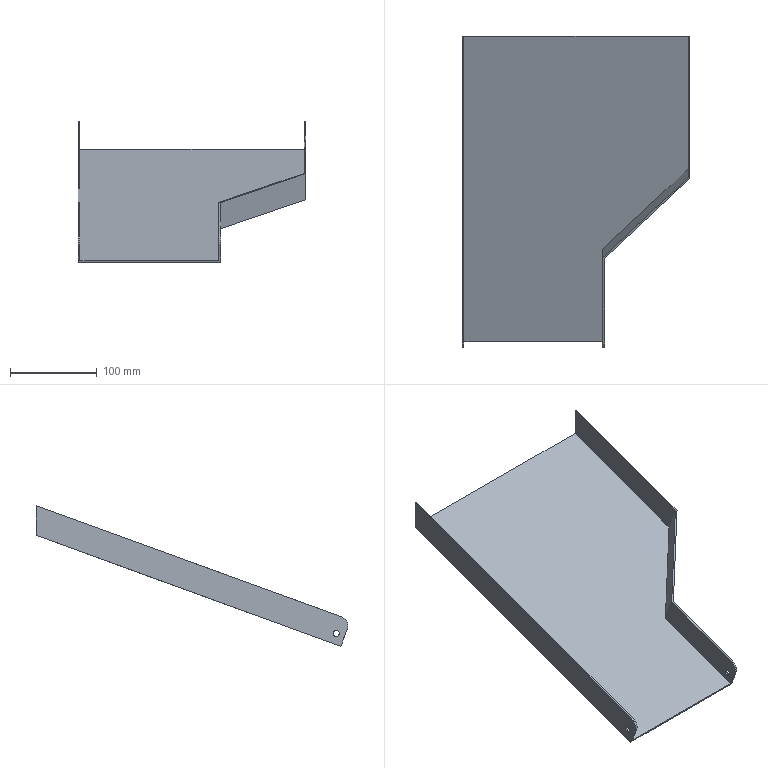Part | NX | features HB 2 | 1 solid | 18 faces | box 262 x 359.033 x 161.773 mm | volume 211954 mm3 | plane 14 | cylinder 4 | commonest cylinder face diameters 7 x2 20 x2
STEP:
#1=CARTESIAN_POINT('',(122.,-585.061,-351.381));
#2=VERTEX_POINT('',#1);
#3=CARTESIAN_POINT('',(122.,-691.589,-390.154));
#4=VERTEX_POINT('',#3);
#5=CARTESIAN_POINT('',(122.,-379.611,-276.603));
#6=DIRECTION('',(0.,-0.9397,-0.342));
#7=VECTOR('',#6,1000.);
#8=LINE('',#5,#7);
#9=EDGE_CURVE('',#2,#4,#8,.T.);
#10=ORIENTED_EDGE('',*,*,#9,.F.);
#11=CARTESIAN_POINT('',(220.,-492.971,-317.863));
#12=VERTEX_POINT('',#11);
#13=CARTESIAN_POINT('',(261.318,-454.145,-303.731));
#14=DIRECTION('',(-0.7071,-0.6645,-0.2418));
#15=VECTOR('',#14,1000.);
#16=LINE('',#13,#15);
#17=EDGE_CURVE('',#12,#2,#16,.T.);
#18=ORIENTED_EDGE('',*,*,#17,.F.);
#19=CARTESIAN_POINT('',(220.,-340.,-262.186));
#20=VERTEX_POINT('',#19);
#21=CARTESIAN_POINT('',(220.,-379.611,-276.603));
#22=DIRECTION('',(0.,-0.9397,-0.342));
#23=VECTOR('',#22,1000.);
#24=LINE('',#21,#23);
#25=EDGE_CURVE('',#20,#12,#24,.T.);
#26=ORIENTED_EDGE('',*,*,#25,.F.);
#27=CARTESIAN_POINT('',(-38.,-340.,-262.186));
#28=VERTEX_POINT('',#27);
#29=CARTESIAN_POINT('',(182.,-340.,-262.186));
#30=DIRECTION('',(-1.,0.,0.));
#31=VECTOR('',#30,1000.);
#32=LINE('',#29,#31);
#33=EDGE_CURVE('',#20,#28,#32,.T.);
#34=ORIENTED_EDGE('',*,*,#33,.T.);
#35=CARTESIAN_POINT('',(-38.,-691.589,-390.154));
#36=VERTEX_POINT('',#35);
#37=CARTESIAN_POINT('',(-38.,-379.611,-276.603));
#38=DIRECTION('',(0.,0.9397,0.342));
#39=VECTOR('',#38,1000.);
#40=LINE('',#37,#39);
#41=EDGE_CURVE('',#36,#28,#40,.T.);
#42=ORIENTED_EDGE('',*,*,#41,.F.);
#43=CARTESIAN_POINT('',(182.,-691.589,-390.154));
#44=DIRECTION('',(1.,0.,0.));
#45=VECTOR('',#44,1000.);
#46=LINE('',#43,#45);
#47=EDGE_CURVE('',#36,#4,#46,.T.);
#48=ORIENTED_EDGE('',*,*,#47,.T.);
#49=EDGE_LOOP('',(#10,#18,#26,#34,#42,#48));
#50=FACE_BOUND('',#49,.T.);
#51=CARTESIAN_POINT('',(182.,-379.611,-276.603));
#52=DIRECTION('',(0.,-0.342,0.9397));
#53=DIRECTION('',(-1.,0.,0.));
#54=AXIS2_PLACEMENT_3D('',#51,#52,#53);
#55=PLANE('',#54);
#56=ADVANCED_FACE('',(#50),#55,.T.);
#57=CARTESIAN_POINT('',(220.,-340.,-230.26));
#58=VERTEX_POINT('',#57);
#59=CARTESIAN_POINT('',(222.,-340.,-230.26));
#60=VERTEX_POINT('',#59);
#61=CARTESIAN_POINT('',(222.,-340.,-230.26));
#62=DIRECTION('',(1.,0.,0.));
#63=VECTOR('',#62,1000.);
#64=LINE('',#61,#63);
#65=EDGE_CURVE('',#58,#60,#64,.T.);
#66=ORIENTED_EDGE('',*,*,#65,.T.);
#67=CARTESIAN_POINT('',(222.,-340.,-264.314));
#68=VERTEX_POINT('',#67);
#69=CARTESIAN_POINT('',(222.,-340.,-276.603));
#70=DIRECTION('',(0.,0.,-1.));
#71=VECTOR('',#70,1000.);
#72=LINE('',#69,#71);
#73=EDGE_CURVE('',#60,#68,#72,.T.);
#74=ORIENTED_EDGE('',*,*,#73,.T.);
#75=CARTESIAN_POINT('',(-40.,-340.,-264.314));
#76=VERTEX_POINT('',#75);
#77=CARTESIAN_POINT('',(182.,-340.,-264.314));
#78=DIRECTION('',(-1.,0.,0.));
#79=VECTOR('',#78,1000.);
#80=LINE('',#77,#79);
#81=EDGE_CURVE('',#68,#76,#80,.T.);
#82=ORIENTED_EDGE('',*,*,#81,.T.);
#83=CARTESIAN_POINT('',(-40.,-340.,-230.26));
#84=VERTEX_POINT('',#83);
#85=CARTESIAN_POINT('',(-40.,-340.,-276.603));
#86=DIRECTION('',(0.,0.,1.));
#87=VECTOR('',#86,1000.);
#88=LINE('',#85,#87);
#89=EDGE_CURVE('',#76,#84,#88,.T.);
#90=ORIENTED_EDGE('',*,*,#89,.T.);
#91=CARTESIAN_POINT('',(-38.,-340.,-230.26));
#92=VERTEX_POINT('',#91);
#93=CARTESIAN_POINT('',(-48.,-340.,-230.26));
#94=DIRECTION('',(1.,0.,0.));
#95=VECTOR('',#94,1000.);
#96=LINE('',#93,#95);
#97=EDGE_CURVE('',#84,#92,#96,.T.);
#98=ORIENTED_EDGE('',*,*,#97,.T.);
#99=CARTESIAN_POINT('',(-38.,-340.,-276.603));
#100=DIRECTION('',(0.,0.,1.));
#101=VECTOR('',#100,1000.);
#102=LINE('',#99,#101);
#103=EDGE_CURVE('',#28,#92,#102,.T.);
#104=ORIENTED_EDGE('',*,*,#103,.F.);
#105=ORIENTED_EDGE('',*,*,#33,.F.);
#106=CARTESIAN_POINT('',(220.,-340.,-276.603));
#107=DIRECTION('',(0.,0.,-1.));
#108=VECTOR('',#107,1000.);
#109=LINE('',#106,#108);
#110=EDGE_CURVE('',#58,#20,#109,.T.);
#111=ORIENTED_EDGE('',*,*,#110,.F.);
#112=EDGE_LOOP('',(#66,#74,#82,#90,#98,#104,#105,#111));
#113=FACE_BOUND('',#112,.T.);
#114=CARTESIAN_POINT('',(-210.,-340.,60.));
#115=DIRECTION('',(0.,1.,0.));
#116=DIRECTION('',(0.,0.,-1.));
#117=AXIS2_PLACEMENT_3D('',#114,#115,#116);
#118=PLANE('',#117);
#119=ADVANCED_FACE('',(#113),#118,.T.);
#120=CARTESIAN_POINT('',(220.,-503.232,-289.672));
#121=VERTEX_POINT('',#120);
#122=CARTESIAN_POINT('',(220.,-492.971,-317.863));
#123=DIRECTION('',(0.,0.342,-0.9397));
#124=VECTOR('',#123,1000.);
#125=LINE('',#122,#124);
#126=EDGE_CURVE('',#121,#12,#125,.T.);
#127=ORIENTED_EDGE('',*,*,#126,.F.);
#128=CARTESIAN_POINT('',(220.,-389.872,-248.412));
#129=DIRECTION('',(0.,-0.9397,-0.342));
#130=VECTOR('',#129,1000.);
#131=LINE('',#128,#130);
#132=EDGE_CURVE('',#58,#121,#131,.T.);
#133=ORIENTED_EDGE('',*,*,#132,.F.);
#134=ORIENTED_EDGE('',*,*,#110,.T.);
#135=ORIENTED_EDGE('',*,*,#25,.T.);
#136=EDGE_LOOP('',(#127,#133,#134,#135));
#137=FACE_BOUND('',#136,.T.);
#138=CARTESIAN_POINT('',(220.,-379.611,-276.603));
#139=DIRECTION('',(-1.,0.,0.));
#140=DIRECTION('',(0.,0.08716,0.9962));
#141=AXIS2_PLACEMENT_3D('',#138,#139,#140);
#142=PLANE('',#141);
#143=ADVANCED_FACE('',(#137),#142,.T.);
#144=CARTESIAN_POINT('',(-40.,-690.905,-392.033));
#145=VERTEX_POINT('',#144);
#146=CARTESIAN_POINT('',(-40.,-378.927,-278.482));
#147=DIRECTION('',(0.,-0.9397,-0.342));
#148=VECTOR('',#147,1000.);
#149=LINE('',#146,#148);
#150=EDGE_CURVE('',#76,#145,#149,.T.);
#151=ORIENTED_EDGE('',*,*,#150,.T.);
#152=CARTESIAN_POINT('',(-40.,-698.43,-371.36));
#153=VERTEX_POINT('',#152);
#154=CARTESIAN_POINT('',(-40.,-691.589,-390.154));
#155=DIRECTION('',(0.,0.342,-0.9397));
#156=VECTOR('',#155,1000.);
#157=LINE('',#154,#156);
#158=EDGE_CURVE('',#153,#145,#157,.T.);
#159=ORIENTED_EDGE('',*,*,#158,.F.);
#160=CARTESIAN_POINT('',(-40.,-692.453,-358.543));
#161=VERTEX_POINT('',#160);
#162=CARTESIAN_POINT('',(-40.,-689.033,-367.939));
#163=DIRECTION('',(-1.,0.,0.));
#164=DIRECTION('',(0.,0.,-1.));
#165=AXIS2_PLACEMENT_3D('',#162,#163,#164);
#166=CIRCLE('',#165,10.);
#167=EDGE_CURVE('',#153,#161,#166,.T.);
#168=ORIENTED_EDGE('',*,*,#167,.T.);
#169=CARTESIAN_POINT('',(-40.,-389.872,-248.412));
#170=DIRECTION('',(0.,-0.9397,-0.342));
#171=VECTOR('',#170,1000.);
#172=LINE('',#169,#171);
#173=EDGE_CURVE('',#84,#161,#172,.T.);
#174=ORIENTED_EDGE('',*,*,#173,.F.);
#175=ORIENTED_EDGE('',*,*,#89,.F.);
#176=EDGE_LOOP('',(#151,#159,#168,#174,#175));
#177=FACE_BOUND('',#176,.T.);
#178=CARTESIAN_POINT('',(-40.,-685.612,-380.836));
#179=VERTEX_POINT('',#178);
#180=CARTESIAN_POINT('',(-40.,-685.612,-377.336));
#181=DIRECTION('',(1.,0.,0.));
#182=DIRECTION('',(0.,0.,-1.));
#183=AXIS2_PLACEMENT_3D('',#180,#181,#182);
#184=CIRCLE('',#183,3.5);
#185=EDGE_CURVE('',#179,#179,#184,.T.);
#186=ORIENTED_EDGE('',*,*,#185,.T.);
#187=EDGE_LOOP('',(#186));
#188=FACE_BOUND('',#187,.T.);
#189=CARTESIAN_POINT('',(-40.,-379.611,-276.603));
#190=DIRECTION('',(1.,0.,0.));
#191=DIRECTION('',(0.,0.08716,0.9962));
#192=AXIS2_PLACEMENT_3D('',#189,#190,#191);
#193=PLANE('',#192);
#194=ADVANCED_FACE('',(#177,#188),#193,.F.);
#195=ORIENTED_EDGE('',*,*,#173,.T.);
#196=CARTESIAN_POINT('',(-38.,-692.453,-358.543));
#197=VERTEX_POINT('',#196);
#198=CARTESIAN_POINT('',(7.,-692.453,-358.543));
#199=DIRECTION('',(1.,0.,0.));
#200=VECTOR('',#199,1000.);
#201=LINE('',#198,#200);
#202=EDGE_CURVE('',#161,#197,#201,.T.);
#203=ORIENTED_EDGE('',*,*,#202,.T.);
#204=CARTESIAN_POINT('',(-38.,-389.872,-248.412));
#205=DIRECTION('',(0.,-0.9397,-0.342));
#206=VECTOR('',#205,1000.);
#207=LINE('',#204,#206);
#208=EDGE_CURVE('',#92,#197,#207,.T.);
#209=ORIENTED_EDGE('',*,*,#208,.F.);
#210=ORIENTED_EDGE('',*,*,#97,.F.);
#211=EDGE_LOOP('',(#195,#203,#209,#210));
#212=FACE_BOUND('',#211,.T.);
#213=CARTESIAN_POINT('',(-48.,-389.872,-248.412));
#214=DIRECTION('',(0.,0.342,-0.9397));
#215=DIRECTION('',(0.,-0.9397,-0.342));
#216=AXIS2_PLACEMENT_3D('',#213,#214,#215);
#217=PLANE('',#216);
#218=ADVANCED_FACE('',(#212),#217,.F.);
#219=CARTESIAN_POINT('',(222.,-493.066,-320.025));
#220=VERTEX_POINT('',#219);
#221=CARTESIAN_POINT('',(124.,-585.156,-353.543));
#222=VERTEX_POINT('',#221);
#223=CARTESIAN_POINT('',(262.732,-454.79,-306.094));
#224=DIRECTION('',(-0.7071,-0.6645,-0.2418));
#225=VECTOR('',#224,1000.);
#226=LINE('',#223,#225);
#227=EDGE_CURVE('',#220,#222,#226,.T.);
#228=ORIENTED_EDGE('',*,*,#227,.T.);
#229=CARTESIAN_POINT('',(124.,-690.905,-392.033));
#230=VERTEX_POINT('',#229);
#231=CARTESIAN_POINT('',(124.,-378.927,-278.482));
#232=DIRECTION('',(0.,0.9397,0.342));
#233=VECTOR('',#232,1000.);
#234=LINE('',#231,#233);
#235=EDGE_CURVE('',#230,#222,#234,.T.);
#236=ORIENTED_EDGE('',*,*,#235,.F.);
#237=CARTESIAN_POINT('',(182.,-690.905,-392.033));
#238=DIRECTION('',(1.,0.,0.));
#239=VECTOR('',#238,1000.);
#240=LINE('',#237,#239);
#241=EDGE_CURVE('',#145,#230,#240,.T.);
#242=ORIENTED_EDGE('',*,*,#241,.F.);
#243=ORIENTED_EDGE('',*,*,#150,.F.);
#244=ORIENTED_EDGE('',*,*,#81,.F.);
#245=CARTESIAN_POINT('',(222.,-378.927,-278.482));
#246=DIRECTION('',(0.,0.9397,0.342));
#247=VECTOR('',#246,1000.);
#248=LINE('',#245,#247);
#249=EDGE_CURVE('',#220,#68,#248,.T.);
#250=ORIENTED_EDGE('',*,*,#249,.F.);
#251=EDGE_LOOP('',(#228,#236,#242,#243,#244,#250));
#252=FACE_BOUND('',#251,.T.);
#253=CARTESIAN_POINT('',(182.,-378.927,-278.482));
#254=DIRECTION('',(0.,-0.342,0.9397));
#255=DIRECTION('',(-1.,0.,0.));
#256=AXIS2_PLACEMENT_3D('',#253,#254,#255);
#257=PLANE('',#256);
#258=ADVANCED_FACE('',(#252),#257,.F.);
#259=CARTESIAN_POINT('',(222.,-504.01,-289.955));
#260=VERTEX_POINT('',#259);
#261=CARTESIAN_POINT('',(222.,-504.01,-289.955));
#262=DIRECTION('',(0.,-0.342,0.9397));
#263=VECTOR('',#262,1000.);
#264=LINE('',#261,#263);
#265=EDGE_CURVE('',#220,#260,#264,.T.);
#266=ORIENTED_EDGE('',*,*,#265,.F.);
#267=ORIENTED_EDGE('',*,*,#249,.T.);
#268=ORIENTED_EDGE('',*,*,#73,.F.);
#269=CARTESIAN_POINT('',(222.,-389.872,-248.412));
#270=DIRECTION('',(0.,-0.9397,-0.342));
#271=VECTOR('',#270,1000.);
#272=LINE('',#269,#271);
#273=EDGE_CURVE('',#60,#260,#272,.T.);
#274=ORIENTED_EDGE('',*,*,#273,.T.);
#275=EDGE_LOOP('',(#266,#267,#268,#274));
#276=FACE_BOUND('',#275,.T.);
#277=CARTESIAN_POINT('',(222.,-379.611,-276.603));
#278=DIRECTION('',(-1.,0.,0.));
#279=DIRECTION('',(0.,-0.08716,-0.9962));
#280=AXIS2_PLACEMENT_3D('',#277,#278,#279);
#281=PLANE('',#280);
#282=ADVANCED_FACE('',(#276),#281,.F.);
#283=CARTESIAN_POINT('',(124.,-596.1,-323.473));
#284=VERTEX_POINT('',#283);
#285=CARTESIAN_POINT('',(282.732,-446.941,-269.184));
#286=DIRECTION('',(0.7071,0.6645,0.2418));
#287=VECTOR('',#286,1000.);
#288=LINE('',#285,#287);
#289=EDGE_CURVE('',#284,#260,#288,.T.);
#290=ORIENTED_EDGE('',*,*,#289,.T.);
#291=ORIENTED_EDGE('',*,*,#273,.F.);
#292=ORIENTED_EDGE('',*,*,#65,.F.);
#293=ORIENTED_EDGE('',*,*,#132,.T.);
#294=CARTESIAN_POINT('',(122.,-595.322,-323.19));
#295=VERTEX_POINT('',#294);
#296=CARTESIAN_POINT('',(281.318,-445.612,-268.7));
#297=DIRECTION('',(0.7071,0.6645,0.2418));
#298=VECTOR('',#297,1000.);
#299=LINE('',#296,#298);
#300=EDGE_CURVE('',#295,#121,#299,.T.);
#301=ORIENTED_EDGE('',*,*,#300,.F.);
#302=CARTESIAN_POINT('',(122.,-692.453,-358.543));
#303=VERTEX_POINT('',#302);
#304=CARTESIAN_POINT('',(122.,-389.872,-248.412));
#305=DIRECTION('',(0.,-0.9397,-0.342));
#306=VECTOR('',#305,1000.);
#307=LINE('',#304,#306);
#308=EDGE_CURVE('',#295,#303,#307,.T.);
#309=ORIENTED_EDGE('',*,*,#308,.T.);
#310=CARTESIAN_POINT('',(124.,-692.453,-358.543));
#311=VERTEX_POINT('',#310);
#312=CARTESIAN_POINT('',(222.,-692.453,-358.543));
#313=DIRECTION('',(1.,0.,0.));
#314=VECTOR('',#313,1000.);
#315=LINE('',#312,#314);
#316=EDGE_CURVE('',#303,#311,#315,.T.);
#317=ORIENTED_EDGE('',*,*,#316,.T.);
#318=CARTESIAN_POINT('',(124.,-389.872,-248.412));
#319=DIRECTION('',(0.,-0.9397,-0.342));
#320=VECTOR('',#319,1000.);
#321=LINE('',#318,#320);
#322=EDGE_CURVE('',#284,#311,#321,.T.);
#323=ORIENTED_EDGE('',*,*,#322,.F.);
#324=EDGE_LOOP('',(#290,#291,#292,#293,#301,#309,#317,#323));
#325=FACE_BOUND('',#324,.T.);
#326=CARTESIAN_POINT('',(222.,-389.872,-248.412));
#327=DIRECTION('',(0.,0.342,-0.9397));
#328=DIRECTION('',(0.,-0.9397,-0.342));
#329=AXIS2_PLACEMENT_3D('',#326,#327,#328);
#330=PLANE('',#329);
#331=ADVANCED_FACE('',(#325),#330,.F.);
#332=ORIENTED_EDGE('',*,*,#208,.T.);
#333=CARTESIAN_POINT('',(-38.,-698.43,-371.36));
#334=VERTEX_POINT('',#333);
#335=CARTESIAN_POINT('',(-38.,-689.033,-367.939));
#336=DIRECTION('',(1.,0.,0.));
#337=DIRECTION('',(0.,0.,-1.));
#338=AXIS2_PLACEMENT_3D('',#335,#336,#337);
#339=CIRCLE('',#338,10.);
#340=EDGE_CURVE('',#197,#334,#339,.T.);
#341=ORIENTED_EDGE('',*,*,#340,.T.);
#342=CARTESIAN_POINT('',(-38.,-691.589,-390.154));
#343=DIRECTION('',(0.,0.342,-0.9397));
#344=VECTOR('',#343,1000.);
#345=LINE('',#342,#344);
#346=EDGE_CURVE('',#334,#36,#345,.T.);
#347=ORIENTED_EDGE('',*,*,#346,.T.);
#348=ORIENTED_EDGE('',*,*,#41,.T.);
#349=ORIENTED_EDGE('',*,*,#103,.T.);
#350=EDGE_LOOP('',(#332,#341,#347,#348,#349));
#351=FACE_BOUND('',#350,.T.);
#352=CARTESIAN_POINT('',(-38.,-685.612,-380.836));
#353=VERTEX_POINT('',#352);
#354=CARTESIAN_POINT('',(-38.,-685.612,-377.336));
#355=DIRECTION('',(-1.,0.,0.));
#356=DIRECTION('',(0.,0.,-1.));
#357=AXIS2_PLACEMENT_3D('',#354,#355,#356);
#358=CIRCLE('',#357,3.5);
#359=EDGE_CURVE('',#353,#353,#358,.T.);
#360=ORIENTED_EDGE('',*,*,#359,.T.);
#361=EDGE_LOOP('',(#360));
#362=FACE_BOUND('',#361,.T.);
#363=CARTESIAN_POINT('',(-38.,-379.611,-276.603));
#364=DIRECTION('',(1.,0.,0.));
#365=DIRECTION('',(0.,0.08716,0.9962));
#366=AXIS2_PLACEMENT_3D('',#363,#364,#365);
#367=PLANE('',#366);
#368=ADVANCED_FACE('',(#351,#362),#367,.T.);
#369=ORIENTED_EDGE('',*,*,#308,.F.);
#370=CARTESIAN_POINT('',(122.,-585.061,-351.381));
#371=DIRECTION('',(0.,-0.342,0.9397));
#372=VECTOR('',#371,1000.);
#373=LINE('',#370,#372);
#374=EDGE_CURVE('',#2,#295,#373,.T.);
#375=ORIENTED_EDGE('',*,*,#374,.F.);
#376=ORIENTED_EDGE('',*,*,#9,.T.);
#377=CARTESIAN_POINT('',(122.,-698.43,-371.36));
#378=VERTEX_POINT('',#377);
#379=CARTESIAN_POINT('',(122.,-691.589,-390.154));
#380=DIRECTION('',(0.,0.342,-0.9397));
#381=VECTOR('',#380,1000.);
#382=LINE('',#379,#381);
#383=EDGE_CURVE('',#378,#4,#382,.T.);
#384=ORIENTED_EDGE('',*,*,#383,.F.);
#385=CARTESIAN_POINT('',(122.,-689.033,-367.939));
#386=DIRECTION('',(-1.,0.,0.));
#387=DIRECTION('',(0.,0.08716,0.9962));
#388=AXIS2_PLACEMENT_3D('',#385,#386,#387);
#389=CIRCLE('',#388,10.);
#390=EDGE_CURVE('',#378,#303,#389,.T.);
#391=ORIENTED_EDGE('',*,*,#390,.T.);
#392=EDGE_LOOP('',(#369,#375,#376,#384,#391));
#393=FACE_BOUND('',#392,.T.);
#394=CARTESIAN_POINT('',(122.,-685.307,-373.85));
#395=VERTEX_POINT('',#394);
#396=CARTESIAN_POINT('',(122.,-685.612,-377.336));
#397=DIRECTION('',(1.,0.,0.));
#398=DIRECTION('',(0.,0.08716,0.9962));
#399=AXIS2_PLACEMENT_3D('',#396,#397,#398);
#400=CIRCLE('',#399,3.5);
#401=EDGE_CURVE('',#395,#395,#400,.T.);
#402=ORIENTED_EDGE('',*,*,#401,.T.);
#403=EDGE_LOOP('',(#402));
#404=FACE_BOUND('',#403,.T.);
#405=CARTESIAN_POINT('',(122.,-379.611,-276.603));
#406=DIRECTION('',(-1.,0.,0.));
#407=DIRECTION('',(0.,0.08716,0.9962));
#408=AXIS2_PLACEMENT_3D('',#405,#406,#407);
#409=PLANE('',#408);
#410=ADVANCED_FACE('',(#393,#404),#409,.T.);
#411=CARTESIAN_POINT('',(124.,-685.307,-373.85));
#412=VERTEX_POINT('',#411);
#413=CARTESIAN_POINT('',(124.,-685.612,-377.336));
#414=DIRECTION('',(1.,0.,0.));
#415=DIRECTION('',(0.,0.08716,0.9962));
#416=AXIS2_PLACEMENT_3D('',#413,#414,#415);
#417=CIRCLE('',#416,3.5);
#418=EDGE_CURVE('',#412,#412,#417,.T.);
#419=ORIENTED_EDGE('',*,*,#418,.F.);
#420=EDGE_LOOP('',(#419));
#421=FACE_BOUND('',#420,.T.);
#422=ORIENTED_EDGE('',*,*,#235,.T.);
#423=CARTESIAN_POINT('',(124.,-596.1,-323.473));
#424=DIRECTION('',(0.,-0.342,0.9397));
#425=VECTOR('',#424,1000.);
#426=LINE('',#423,#425);
#427=EDGE_CURVE('',#222,#284,#426,.T.);
#428=ORIENTED_EDGE('',*,*,#427,.T.);
#429=ORIENTED_EDGE('',*,*,#322,.T.);
#430=CARTESIAN_POINT('',(124.,-698.43,-371.36));
#431=VERTEX_POINT('',#430);
#432=CARTESIAN_POINT('',(124.,-689.033,-367.939));
#433=DIRECTION('',(1.,0.,0.));
#434=DIRECTION('',(0.,0.08716,0.9962));
#435=AXIS2_PLACEMENT_3D('',#432,#433,#434);
#436=CIRCLE('',#435,10.);
#437=EDGE_CURVE('',#311,#431,#436,.T.);
#438=ORIENTED_EDGE('',*,*,#437,.T.);
#439=CARTESIAN_POINT('',(124.,-691.589,-390.154));
#440=DIRECTION('',(0.,0.342,-0.9397));
#441=VECTOR('',#440,1000.);
#442=LINE('',#439,#441);
#443=EDGE_CURVE('',#431,#230,#442,.T.);
#444=ORIENTED_EDGE('',*,*,#443,.T.);
#445=EDGE_LOOP('',(#422,#428,#429,#438,#444));
#446=FACE_BOUND('',#445,.T.);
#447=CARTESIAN_POINT('',(124.,-379.611,-276.603));
#448=DIRECTION('',(-1.,0.,0.));
#449=DIRECTION('',(0.,-0.08716,-0.9962));
#450=AXIS2_PLACEMENT_3D('',#447,#448,#449);
#451=PLANE('',#450);
#452=ADVANCED_FACE('',(#421,#446),#451,.F.);
#453=ORIENTED_EDGE('',*,*,#401,.F.);
#454=EDGE_LOOP('',(#453));
#455=FACE_BOUND('',#454,.T.);
#456=ORIENTED_EDGE('',*,*,#418,.T.);
#457=EDGE_LOOP('',(#456));
#458=FACE_BOUND('',#457,.T.);
#459=CARTESIAN_POINT('',(826.,-685.612,-377.336));
#460=DIRECTION('',(-1.,0.,0.));
#461=DIRECTION('',(0.,-0.08716,-0.9962));
#462=AXIS2_PLACEMENT_3D('',#459,#460,#461);
#463=CYLINDRICAL_SURFACE('',#462,3.5);
#464=ADVANCED_FACE('',(#455,#458),#463,.F.);
#465=ORIENTED_EDGE('',*,*,#390,.F.);
#466=CARTESIAN_POINT('',(182.,-698.43,-371.36));
#467=DIRECTION('',(-1.,0.,0.));
#468=VECTOR('',#467,1000.);
#469=LINE('',#466,#468);
#470=EDGE_CURVE('',#431,#378,#469,.T.);
#471=ORIENTED_EDGE('',*,*,#470,.F.);
#472=ORIENTED_EDGE('',*,*,#437,.F.);
#473=ORIENTED_EDGE('',*,*,#316,.F.);
#474=EDGE_LOOP('',(#465,#471,#472,#473));
#475=FACE_BOUND('',#474,.T.);
#476=CARTESIAN_POINT('',(222.,-689.033,-367.939));
#477=DIRECTION('',(1.,0.,0.));
#478=DIRECTION('',(0.,0.08716,0.9962));
#479=AXIS2_PLACEMENT_3D('',#476,#477,#478);
#480=CYLINDRICAL_SURFACE('',#479,10.);
#481=ADVANCED_FACE('',(#475),#480,.T.);
#482=ORIENTED_EDGE('',*,*,#47,.F.);
#483=ORIENTED_EDGE('',*,*,#346,.F.);
#484=CARTESIAN_POINT('',(265.,-698.43,-371.36));
#485=DIRECTION('',(-1.,0.,0.));
#486=VECTOR('',#485,1000.);
#487=LINE('',#484,#486);
#488=EDGE_CURVE('',#334,#153,#487,.T.);
#489=ORIENTED_EDGE('',*,*,#488,.T.);
#490=ORIENTED_EDGE('',*,*,#158,.T.);
#491=ORIENTED_EDGE('',*,*,#241,.T.);
#492=ORIENTED_EDGE('',*,*,#443,.F.);
#493=ORIENTED_EDGE('',*,*,#470,.T.);
#494=ORIENTED_EDGE('',*,*,#383,.T.);
#495=EDGE_LOOP('',(#482,#483,#489,#490,#491,#492,#493,#494));
#496=FACE_BOUND('',#495,.T.);
#497=CARTESIAN_POINT('',(182.,-691.589,-390.154));
#498=DIRECTION('',(0.,0.9397,0.342));
#499=DIRECTION('',(0.,0.342,-0.9397));
#500=AXIS2_PLACEMENT_3D('',#497,#498,#499);
#501=PLANE('',#500);
#502=ADVANCED_FACE('',(#496),#501,.F.);
#503=ORIENTED_EDGE('',*,*,#340,.F.);
#504=ORIENTED_EDGE('',*,*,#202,.F.);
#505=ORIENTED_EDGE('',*,*,#167,.F.);
#506=ORIENTED_EDGE('',*,*,#488,.F.);
#507=EDGE_LOOP('',(#503,#504,#505,#506));
#508=FACE_BOUND('',#507,.T.);
#509=CARTESIAN_POINT('',(265.,-689.033,-367.939));
#510=DIRECTION('',(-1.,0.,0.));
#511=DIRECTION('',(0.,-0.08716,-0.9962));
#512=AXIS2_PLACEMENT_3D('',#509,#510,#511);
#513=CYLINDRICAL_SURFACE('',#512,10.);
#514=ADVANCED_FACE('',(#508),#513,.T.);
#515=ORIENTED_EDGE('',*,*,#359,.F.);
#516=EDGE_LOOP('',(#515));
#517=FACE_BOUND('',#516,.T.);
#518=ORIENTED_EDGE('',*,*,#185,.F.);
#519=EDGE_LOOP('',(#518));
#520=FACE_BOUND('',#519,.T.);
#521=CARTESIAN_POINT('',(857.,-685.612,-377.336));
#522=DIRECTION('',(-1.,0.,0.));
#523=DIRECTION('',(0.,-0.08716,-0.9962));
#524=AXIS2_PLACEMENT_3D('',#521,#522,#523);
#525=CYLINDRICAL_SURFACE('',#524,3.5);
#526=ADVANCED_FACE('',(#517,#520),#525,.F.);
#527=ORIENTED_EDGE('',*,*,#427,.F.);
#528=ORIENTED_EDGE('',*,*,#227,.F.);
#529=ORIENTED_EDGE('',*,*,#265,.T.);
#530=ORIENTED_EDGE('',*,*,#289,.F.);
#531=EDGE_LOOP('',(#527,#528,#529,#530));
#532=FACE_BOUND('',#531,.T.);
#533=CARTESIAN_POINT('',(224.,-502.131,-289.271));
#534=DIRECTION('',(-0.7071,0.6645,0.2418));
#535=DIRECTION('',(0.,-0.342,0.9397));
#536=AXIS2_PLACEMENT_3D('',#533,#534,#535);
#537=PLANE('',#536);
#538=ADVANCED_FACE('',(#532),#537,.F.);
#539=ORIENTED_EDGE('',*,*,#126,.T.);
#540=ORIENTED_EDGE('',*,*,#17,.T.);
#541=ORIENTED_EDGE('',*,*,#374,.T.);
#542=ORIENTED_EDGE('',*,*,#300,.T.);
#543=EDGE_LOOP('',(#539,#540,#541,#542));
#544=FACE_BOUND('',#543,.T.);
#545=CARTESIAN_POINT('',(222.586,-500.802,-288.787));
#546=DIRECTION('',(-0.7071,0.6645,0.2418));
#547=DIRECTION('',(0.,-0.342,0.9397));
#548=AXIS2_PLACEMENT_3D('',#545,#546,#547);
#549=PLANE('',#548);
#550=ADVANCED_FACE('',(#544),#549,.T.);
#551=CLOSED_SHELL('',(#56,#119,#143,#194,#218,#258,#282,#331,#368,#410,#452,#464,#481,#502,#514,#526,#538,#550));
#552=MANIFOLD_SOLID_BREP('',#551);
#553=(LENGTH_UNIT()NAMED_UNIT(*)SI_UNIT(.MILLI.,.METRE.));
#554=UNCERTAINTY_MEASURE_WITH_UNIT(LENGTH_MEASURE(0.00001),#553,'','');
#555=(NAMED_UNIT(*)PLANE_ANGLE_UNIT()SI_UNIT($,.RADIAN.));
#556=(NAMED_UNIT(*)SI_UNIT($,.STERADIAN.)SOLID_ANGLE_UNIT());
#557=(GEOMETRIC_REPRESENTATION_CONTEXT(3)GLOBAL_UNCERTAINTY_ASSIGNED_CONTEXT((#554))GLOBAL_UNIT_ASSIGNED_CONTEXT((#553,#555,#556))REPRESENTATION_CONTEXT('',''));
#558=ADVANCED_BREP_SHAPE_REPRESENTATION('',(#552),#557);